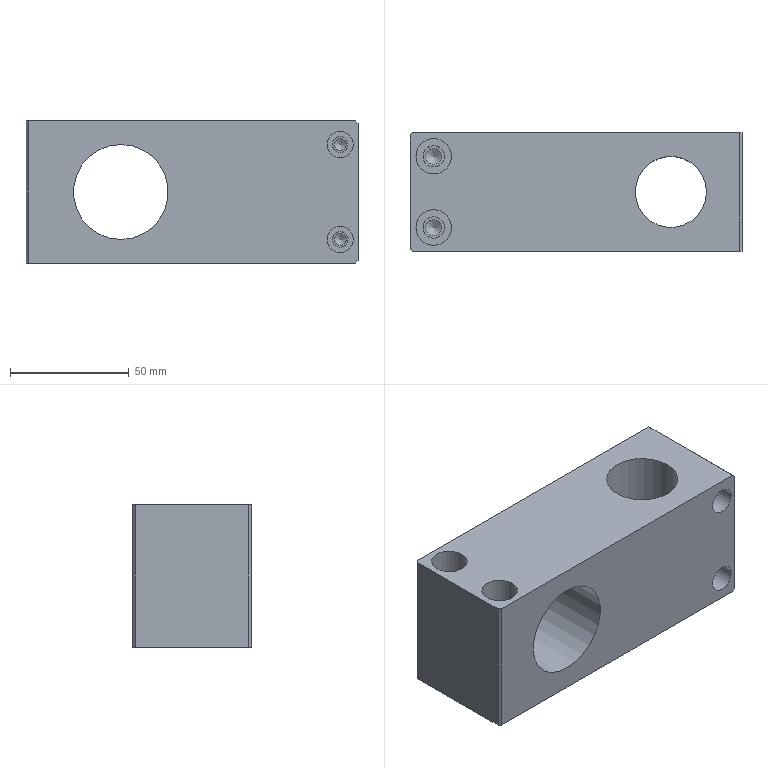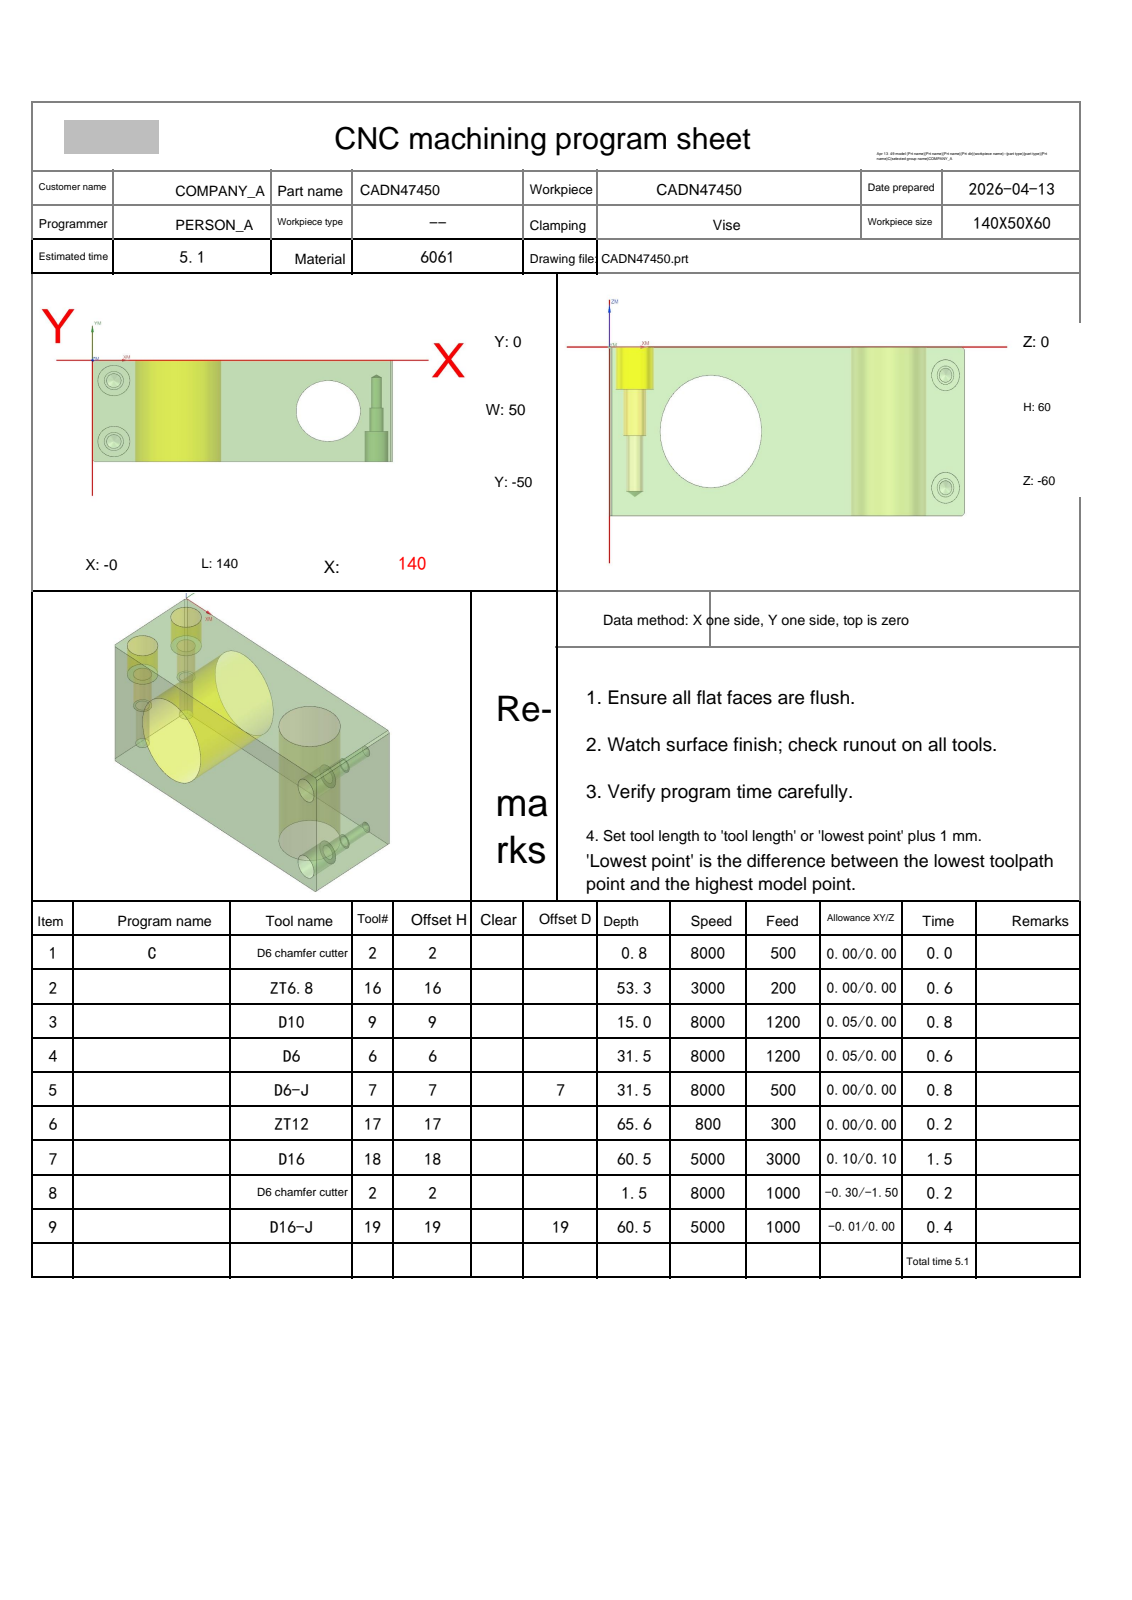NC program | NX | posted by the shop | part box 140 x 50 x 60 mm
Whole program:
%
O0001
(Machine time: 6.89 MIN)
(===Total Tool:8===)
(T2=D6 chamfer cutter   D=6.   R=0.   D-  H02 Z=-1.5  )
(T16=ZT6.8  D=6.8  DR_a=118 D-  H16 Z=-53.29)
(T9=D10     D=10.  R=0.   D-  H09 Z=-15.  )
(T6=D6      D=6.   R=0.   D-  H06 Z=-31.5 )
(T7=D6-J    D=6.   R=0.   D7  H07 Z=-31.5 )
(T17=ZT12   D=12.  DR_a=118 D-  H17 Z=-65.61)
(T18=D16    D=16.  R=0.   D-  H18 Z=-60.5 )
(T19=D16-J  D=16.  R=0.   D19 H19 Z=-60.5 )
G80 G90 G17 G49 G40
G91 G28 Z0
M01
N1 T02 M06
(D6 chamfer cutter  D=6. R=0. H=02 ce=0.00 di=0.00)
G00 G90 G54 X10. Y-40. M03 S8000
G43 H02 Z20.
M08
G98 G81 X10. Y-40. Z-.8 R1. F500.
Y-10.
X110. Y-25.
G80
G00 Z20.
G91 G28 Z0.0
M05
M09
G91 G28 Z0.0
M01
N2 T16 M06
(ZT6.8 D=6.8 DR_a=118 H=16)
G00 G90 G54 X10. Y-40. M03 S3000
G43 H16 Z20.
M08
G98 G83 X10. Y-40. Z-53.293 R1. F200. Q2.
Y-10.
G80
G00 Z20.
G91 G28 Z0.0
M05
M09
G91 G28 Z0.0
M01
N3 T09 M06
(D10  D=10. R=0. H=09 ce=0.05 di=0.00)
G00 G90 G54 X10. Y-40. M03 S8000
G43 H09 Z20.
M08
Z.5
G03 X11.225 Y-41.225 I1.225 J0.0 F1200.
X12.45 Y-40. I0.0 J1.225
X12.45 Y-40. Z0.0 I-2.45 J0.0
X12.45 Y-40. Z-.5 I-2.45 J0.0
X12.45 Y-40. Z-1. I-2.45 J0.0
X12.45 Y-40. Z-1.5 I-2.45 J0.0
X12.45 Y-40. Z-2. I-2.45 J0.0
X12.45 Y-40. Z-2.5 I-2.45 J0.0
X12.45 Y-40. Z-3. I-2.45 J0.0
X12.45 Y-40. Z-3.5 I-2.45 J0.0
X12.45 Y-40. Z-4. I-2.45 J0.0
X12.45 Y-40. Z-4.5 I-2.45 J0.0
X12.45 Y-40. Z-5. I-2.45 J0.0
X12.45 Y-40. Z-5.5 I-2.45 J0.0
X12.45 Y-40. Z-6. I-2.45 J0.0
X12.45 Y-40. Z-6.5 I-2.45 J0.0
X12.45 Y-40. Z-7. I-2.45 J0.0
X12.45 Y-40. Z-7.5 I-2.45 J0.0
X12.45 Y-40. Z-8. I-2.45 J0.0
X12.45 Y-40. Z-8.5 I-2.45 J0.0
X12.45 Y-40. Z-9. I-2.45 J0.0
X12.45 Y-40. Z-9.5 I-2.45 J0.0
X12.45 Y-40. Z-10. I-2.45 J0.0
X12.45 Y-40. Z-10.5 I-2.45 J0.0
X12.45 Y-40. Z-11. I-2.45 J0.0
X12.45 Y-40. Z-11.5 I-2.45 J0.0
X12.45 Y-40. Z-12. I-2.45 J0.0
X12.45 Y-40. Z-12.5 I-2.45 J0.0
X12.45 Y-40. Z-13. I-2.45 J0.0
X12.45 Y-40. Z-13.5 I-2.45 J0.0
X12.45 Y-40. Z-14. I-2.45 J0.0
X12.45 Y-40. Z-14.5 I-2.45 J0.0
X12.45 Y-40. Z-15. I-2.45 J0.0
X10. Y-37.55 I-2.45 J0.0
X7.55 Y-40. I0.0 J-2.45
X10. Y-42.45 I2.45 J0.0
X12.45 Y-40. I0.0 J2.45
X11.225 Y-38.775 I-1.225 J0.0
X10. Y-40. I0.0 J-1.225
G00 Z20.
Y-10.
Z.5
G03 X11.225 Y-11.225 I1.225 J0.0
X12.45 Y-10. I0.0 J1.225
X12.45 Y-10. Z0.0 I-2.45 J0.0
X12.45 Y-10. Z-.5 I-2.45 J0.0
X12.45 Y-10. Z-1. I-2.45 J0.0
X12.45 Y-10. Z-1.5 I-2.45 J0.0
X12.45 Y-10. Z-2. I-2.45 J0.0
X12.45 Y-10. Z-2.5 I-2.45 J0.0
X12.45 Y-10. Z-3. I-2.45 J0.0
X12.45 Y-10. Z-3.5 I-2.45 J0.0
X12.45 Y-10. Z-4. I-2.45 J0.0
X12.45 Y-10. Z-4.5 I-2.45 J0.0
X12.45 Y-10. Z-5. I-2.45 J0.0
X12.45 Y-10. Z-5.5 I-2.45 J0.0
X12.45 Y-10. Z-6. I-2.45 J0.0
X12.45 Y-10. Z-6.5 I-2.45 J0.0
X12.45 Y-10. Z-7. I-2.45 J0.0
X12.45 Y-10. Z-7.5 I-2.45 J0.0
X12.45 Y-10. Z-8. I-2.45 J0.0
X12.45 Y-10. Z-8.5 I-2.45 J0.0
X12.45 Y-10. Z-9. I-2.45 J0.0
X12.45 Y-10. Z-9.5 I-2.45 J0.0
X12.45 Y-10. Z-10. I-2.45 J0.0
X12.45 Y-10. Z-10.5 I-2.45 J0.0
X12.45 Y-10. Z-11. I-2.45 J0.0
X12.45 Y-10. Z-11.5 I-2.45 J0.0
X12.45 Y-10. Z-12. I-2.45 J0.0
X12.45 Y-10. Z-12.5 I-2.45 J0.0
X12.45 Y-10. Z-13. I-2.45 J0.0
X12.45 Y-10. Z-13.5 I-2.45 J0.0
X12.45 Y-10. Z-14. I-2.45 J0.0
X12.45 Y-10. Z-14.5 I-2.45 J0.0
X12.45 Y-10. Z-15. I-2.45 J0.0
X10. Y-7.55 I-2.45 J0.0
X7.55 Y-10. I0.0 J-2.45
X10. Y-12.45 I2.45 J0.0
X12.45 Y-10. I0.0 J2.45
X11.225 Y-8.775 I-1.225 J0.0
X10. Y-10. I0.0 J-1.225
G00 Z20.
G91 G28 Z0.0
M05
M09
G91 G28 Z0.0
M01
N4 T06 M06
(D6  D=6. R=0. H=06 ce=0.05 di=0.00)
G00 G90 G54 X10. Y-40. M03 S8000
G43 H06 Z20.
M08
Z-14.5
G03 X10.725 Y-40.725 I.725 J0.0 F1200.
X11.45 Y-40. I0.0 J.725
X11.45 Y-40. Z-15. I-1.45 J0.0
X11.45 Y-40. Z-15.5 I-1.45 J0.0
X11.45 Y-40. Z-16. I-1.45 J0.0
X11.45 Y-40. Z-16.5 I-1.45 J0.0
X11.45 Y-40. Z-17. I-1.45 J0.0
X11.45 Y-40. Z-17.5 I-1.45 J0.0
X11.45 Y-40. Z-18. I-1.45 J0.0
X11.45 Y-40. Z-18.5 I-1.45 J0.0
X11.45 Y-40. Z-19. I-1.45 J0.0
X11.45 Y-40. Z-19.5 I-1.45 J0.0
X11.45 Y-40. Z-20. I-1.45 J0.0
X11.45 Y-40. Z-20.5 I-1.45 J0.0
X11.45 Y-40. Z-21. I-1.45 J0.0
X11.45 Y-40. Z-21.5 I-1.45 J0.0
X11.45 Y-40. Z-22. I-1.45 J0.0
X11.45 Y-40. Z-22.5 I-1.45 J0.0
X11.45 Y-40. Z-23. I-1.45 J0.0
X11.45 Y-40. Z-23.5 I-1.45 J0.0
X11.45 Y-40. Z-24. I-1.45 J0.0
X11.45 Y-40. Z-24.5 I-1.45 J0.0
X11.45 Y-40. Z-25. I-1.45 J0.0
X11.45 Y-40. Z-25.5 I-1.45 J0.0
X11.45 Y-40. Z-26. I-1.45 J0.0
X11.45 Y-40. Z-26.5 I-1.45 J0.0
X11.45 Y-40. Z-27. I-1.45 J0.0
X11.45 Y-40. Z-27.5 I-1.45 J0.0
X11.45 Y-40. Z-28. I-1.45 J0.0
X11.45 Y-40. Z-28.5 I-1.45 J0.0
X11.45 Y-40. Z-29. I-1.45 J0.0
X11.45 Y-40. Z-29.5 I-1.45 J0.0
X11.45 Y-40. Z-30. I-1.45 J0.0
X11.45 Y-40. Z-30.5 I-1.45 J0.0
X11.45 Y-40. Z-31. I-1.45 J0.0
X11.45 Y-40. Z-31.5 I-1.45 J0.0
X10. Y-38.55 I-1.45 J0.0
X8.55 Y-40. I0.0 J-1.45
X10. Y-41.45 I1.45 J0.0
X11.45 Y-40. I0.0 J1.45
X10.725 Y-39.275 I-.725 J0.0
X10. Y-40. I0.0 J-.725
G00 Z20.
Y-10.
Z-14.5
G03 X10.725 Y-10.725 I.725 J0.0
X11.45 Y-10. I0.0 J.725
X11.45 Y-10. Z-15. I-1.45 J0.0
X11.45 Y-10. Z-15.5 I-1.45 J0.0
X11.45 Y-10. Z-16. I-1.45 J0.0
X11.45 Y-10. Z-16.5 I-1.45 J0.0
X11.45 Y-10. Z-17. I-1.45 J0.0
X11.45 Y-10. Z-17.5 I-1.45 J0.0
X11.45 Y-10. Z-18. I-1.45 J0.0
X11.45 Y-10. Z-18.5 I-1.45 J0.0
X11.45 Y-10. Z-19. I-1.45 J0.0
X11.45 Y-10. Z-19.5 I-1.45 J0.0
X11.45 Y-10. Z-20. I-1.45 J0.0
X11.45 Y-10. Z-20.5 I-1.45 J0.0
X11.45 Y-10. Z-21. I-1.45 J0.0
X11.45 Y-10. Z-21.5 I-1.45 J0.0
X11.45 Y-10. Z-22. I-1.45 J0.0
X11.45 Y-10. Z-22.5 I-1.45 J0.0
X11.45 Y-10. Z-23. I-1.45 J0.0
X11.45 Y-10. Z-23.5 I-1.45 J0.0
X11.45 Y-10. Z-24. I-1.45 J0.0
X11.45 Y-10. Z-24.5 I-1.45 J0.0
X11.45 Y-10. Z-25. I-1.45 J0.0
X11.45 Y-10. Z-25.5 I-1.45 J0.0
X11.45 Y-10. Z-26. I-1.45 J0.0
X11.45 Y-10. Z-26.5 I-1.45 J0.0
X11.45 Y-10. Z-27. I-1.45 J0.0
X11.45 Y-10. Z-27.5 I-1.45 J0.0
X11.45 Y-10. Z-28. I-1.45 J0.0
X11.45 Y-10. Z-28.5 I-1.45 J0.0
X11.45 Y-10. Z-29. I-1.45 J0.0
X11.45 Y-10. Z-29.5 I-1.45 J0.0
X11.45 Y-10. Z-30. I-1.45 J0.0
X11.45 Y-10. Z-30.5 I-1.45 J0.0
X11.45 Y-10. Z-31. I-1.45 J0.0
X11.45 Y-10. Z-31.5 I-1.45 J0.0
X10. Y-8.55 I-1.45 J0.0
X8.55 Y-10. I0.0 J-1.45
X10. Y-11.45 I1.45 J0.0
X11.45 Y-10. I0.0 J1.45
X10.725 Y-9.275 I-.725 J0.0
X10. Y-10. I0.0 J-.725
G00 Z20.
G91 G28 Z0.0
M05
M09
G91 G28 Z0.0
M01
N5 T07 M06
(D6-J  D=6. R=0. H=07 ce=0.00 di=0.00)
G00 G90 G54 X10. Y-40. M03 S8000
G43 H07 Z20.
M08
Z.5
G41 D07
G01 X10.847 Y-41.177 F500.
G03 X12.484 Y-42.016 I1.637 J1.177
X14.5 Y-40. I0.0 J2.016
X14.5 Y-40. Z-4.5 I-4.5 J0.0
X14.5 Y-40. Z-9.5 I-4.5 J0.0
X14.5 Y-40. Z-14.5 I-4.5 J0.0
X13.641 Y-37.355 Z-15. I-4.5 J0.0
X10. Y-35.5 I-3.641 J-2.645
X5.5 Y-40. I0.0 J-4.5
X10. Y-44.5 I4.5 J0.0
X14.5 Y-40. I0.0 J4.5
X13.641 Y-37.355 I-4.5 J0.0
X12.009 Y-36.524 I-1.631 J-1.185
X9.993 Y-38.54 I0.0 J-2.016
G01 Y-38.55
G40 X10. Y-40.
G00 Z20.
Y-10.
Z.5
G41 D07
G01 X10.847 Y-11.177
G03 X12.484 Y-12.016 I1.637 J1.177
X14.5 Y-10. I0.0 J2.016
X14.5 Y-10. Z-4.5 I-4.5 J0.0
X14.5 Y-10. Z-9.5 I-4.5 J0.0
X14.5 Y-10. Z-14.5 I-4.5 J0.0
X13.641 Y-7.355 Z-15. I-4.5 J0.0
X10. Y-5.5 I-3.641 J-2.645
X5.5 Y-10. I0.0 J-4.5
X10. Y-14.5 I4.5 J0.0
X14.5 Y-10. I0.0 J4.5
X13.641 Y-7.355 I-4.5 J0.0
X12.009 Y-6.524 I-1.631 J-1.185
X9.993 Y-8.54 I0.0 J-2.016
G01 Y-8.55
G40 X10. Y-10.
G00 Z20.
G00 G90 X10. Y-40. M03 S8000
Z20.
Z-14.5
G41 D07
G01 X10.052 Y-40.193 F500.
G03 X10.763 Y-40.737 I.711 J.193
X11.5 Y-40. I0.0 J.737
X11.5 Y-40. Z-19.5 I-1.5 J0.0
X11.5 Y-40. Z-24.5 I-1.5 J0.0
X11.5 Y-40. Z-29.5 I-1.5 J0.0
X8.786 Y-39.118 Z-31.5 I-1.5 J0.0
X8.5 Y-40. I1.214 J-.882
X10. Y-41.5 I1.5 J0.0
X11.5 Y-40. I0.0 J1.5
X10. Y-38.5 I-1.5 J0.0
X8.786 Y-39.118 I0.0 J-1.5
X8.646 Y-39.551 I.596 J-.433
X9.382 Y-40.288 I.737 J0.0
X9.844 Y-40.125 I0.0 J.737
G01 G40 X10. Y-40.
G00 Z20.
Y-10.
Z-14.5
G41 D07
G01 X10.052 Y-10.193
G03 X10.763 Y-10.737 I.711 J.193
X11.5 Y-10. I0.0 J.737
X11.5 Y-10. Z-19.5 I-1.5 J0.0
X11.5 Y-10. Z-24.5 I-1.5 J0.0
X11.5 Y-10. Z-29.5 I-1.5 J0.0
X8.786 Y-9.118 Z-31.5 I-1.5 J0.0
X8.5 Y-10. I1.214 J-.882
X10. Y-11.5 I1.5 J0.0
X11.5 Y-10. I0.0 J1.5
X10. Y-8.5 I-1.5 J0.0
X8.786 Y-9.118 I0.0 J-1.5
X8.646 Y-9.551 I.596 J-.433
X9.382 Y-10.288 I.737 J0.0
X9.844 Y-10.125 I0.0 J.737
G01 G40 X10. Y-10.
G00 Z20.
G91 G28 Z0.0
M05
M09
G91 G28 Z0.0
M01
N6 T17 M06
(ZT12 D=12. DR_a=118 H=17)
G00 G90 G54 X110. Y-25. M03 S800
G43 H17 Z20.
M08
G98 G83 X110. Y-25. Z-65.605 R1. F300. Q3.
G80
G00 Z20.
G91 G28 Z0.0
M05
M09
G91 G28 Z0.0
M01
N7 T18 M06
(D16  D=16. R=0. H=18 ce=0.10 di=0.10)
G00 G90 G54 X112.571 Y-31.398 M03 S5000
G43 H18 Z20.
M08
Z1.
G01 X113.65 Y-30.891 Z.938 F3000.
X114.9 Y-29.9 Z.854
X115.891 Y-28.65 Z.77
X116.57 Y-27.205 Z.687
X116.9 Y-25.644 Z.603
Y-24.356 Z.536
X116.57 Y-22.795 Z.452
X115.891 Y-21.35 Z.368
X114.9 Y-20.1 Z.285
X113.65 Y-19.109 Z.201
X112.205 Y-18.43 Z.117
X110.644 Y-18.1 Z.034
X110. Z0.0
G03 X103.1 Y-25. Z-.15 I0.0 J-6.9
X110. Y-31.9 Z-.3 I6.9 J0.0
X116.9 Y-25. Z-.449 I0.0 J6.9
X110. Y-18.1 Z-.599 I-6.9 J0.0
X103.1 Y-25. Z-.749 I0.0 J-6.9
X110. Y-31.9 Z-.899 I6.9 J0.0
X116.9 Y-25. Z-1.048 I0.0 J6.9
X110. Y-18.1 Z-1.198 I-6.9 J0.0
X103.1 Y-25. Z-1.348 I0.0 J-6.9
X110. Y-31.9 Z-1.498 I6.9 J0.0
X116.9 Y-25. Z-1.647 I0.0 J6.9
X110. Y-18.1 Z-1.797 I-6.9 J0.0
X103.1 Y-25. Z-1.947 I0.0 J-6.9
X110. Y-31.9 Z-2.097 I6.9 J0.0
X116.9 Y-25. Z-2.246 I0.0 J6.9
X110. Y-18.1 Z-2.396 I-6.9 J0.0
X103.1 Y-25. Z-2.546 I0.0 J-6.9
X110. Y-31.9 Z-2.696 I6.9 J0.0
X116.9 Y-25. Z-2.845 I0.0 J6.9
X110. Y-18.1 Z-2.995 I-6.9 J0.0
X103.1 Y-25. Z-3.145 I0.0 J-6.9
X110. Y-31.9 Z-3.295 I6.9 J0.0
X116.9 Y-25. Z-3.444 I0.0 J6.9
X110. Y-18.1 Z-3.594 I-6.9 J0.0
X103.1 Y-25. Z-3.744 I0.0 J-6.9
X110. Y-31.9 Z-3.894 I6.9 J0.0
X116.9 Y-25. Z-4.043 I0.0 J6.9
X110. Y-18.1 Z-4.193 I-6.9 J0.0
X103.1 Y-25. Z-4.343 I0.0 J-6.9
X110. Y-31.9 Z-4.493 I6.9 J0.0
X116.9 Y-25. Z-4.642 I0.0 J6.9
X110. Y-18.1 Z-4.792 I-6.9 J0.0
X103.1 Y-25. Z-4.942 I0.0 J-6.9
X110. Y-31.9 Z-5.092 I6.9 J0.0
X116.9 Y-25. Z-5.241 I0.0 J6.9
X110. Y-18.1 Z-5.391 I-6.9 J0.0
X103.1 Y-25. Z-5.541 I0.0 J-6.9
X110. Y-31.9 Z-5.691 I6.9 J0.0
X116.9 Y-25. Z-5.84 I0.0 J6.9
X110. Y-18.1 Z-5.99 I-6.9 J0.0
X103.1 Y-25. Z-6.14 I0.0 J-6.9
X110. Y-31.9 Z-6.29 I6.9 J0.0
X116.9 Y-25. Z-6.439 I0.0 J6.9
X110. Y-18.1 Z-6.589 I-6.9 J0.0
X103.1 Y-25. Z-6.739 I0.0 J-6.9
X110. Y-31.9 Z-6.889 I6.9 J0.0
X116.9 Y-25. Z-7.038 I0.0 J6.9
X110. Y-18.1 Z-7.188 I-6.9 J0.0
X103.1 Y-25. Z-7.338 I0.0 J-6.9
X110. Y-31.9 Z-7.488 I6.9 J0.0
X116.9 Y-25. Z-7.637 I0.0 J6.9
X110. Y-18.1 Z-7.787 I-6.9 J0.0
X103.1 Y-25. Z-7.937 I0.0 J-6.9
X110. Y-31.9 Z-8.087 I6.9 J0.0
X116.9 Y-25. Z-8.236 I0.0 J6.9
X110. Y-18.1 Z-8.386 I-6.9 J0.0
X103.1 Y-25. Z-8.536 I0.0 J-6.9
X110. Y-31.9 Z-8.686 I6.9 J0.0
X116.9 Y-25. Z-8.835 I0.0 J6.9
X110. Y-18.1 Z-8.985 I-6.9 J0.0
X103.1 Y-25. Z-9.135 I0.0 J-6.9
X110. Y-31.9 Z-9.285 I6.9 J0.0
X116.9 Y-25. Z-9.434 I0.0 J6.9
X110. Y-18.1 Z-9.584 I-6.9 J0.0
X103.1 Y-25. Z-9.734 I0.0 J-6.9
X110. Y-31.9 Z-9.884 I6.9 J0.0
X116.9 Y-25. Z-10.033 I0.0 J6.9
X110. Y-18.1 Z-10.183 I-6.9 J0.0
X103.1 Y-25. Z-10.333 I0.0 J-6.9
X110. Y-31.9 Z-10.483 I6.9 J0.0
X116.9 Y-25. Z-10.632 I0.0 J6.9
X110. Y-18.1 Z-10.782 I-6.9 J0.0
X103.1 Y-25. Z-10.932 I0.0 J-6.9
X110. Y-31.9 Z-11.082 I6.9 J0.0
X116.9 Y-25. Z-11.231 I0.0 J6.9
X110. Y-18.1 Z-11.381 I-6.9 J0.0
X103.1 Y-25. Z-11.531 I0.0 J-6.9
X110. Y-31.9 Z-11.681 I6.9 J0.0
X116.9 Y-25. Z-11.83 I0.0 J6.9
X110. Y-18.1 Z-11.98 I-6.9 J0.0
X103.1 Y-25. Z-12.13 I0.0 J-6.9
X110. Y-31.9 Z-12.28 I6.9 J0.0
X116.9 Y-25. Z-12.429 I0.0 J6.9
X110. Y-18.1 Z-12.579 I-6.9 J0.0
X103.1 Y-25. Z-12.729 I0.0 J-6.9
X110. Y-31.9 Z-12.879 I6.9 J0.0
X116.9 Y-25. Z-13.028 I0.0 J6.9
X110. Y-18.1 Z-13.178 I-6.9 J0.0
X103.1 Y-25. Z-13.328 I0.0 J-6.9
X110. Y-31.9 Z-13.478 I6.9 J0.0
X116.9 Y-25. Z-13.627 I0.0 J6.9
X110. Y-18.1 Z-13.777 I-6.9 J0.0
X103.1 Y-25. Z-13.927 I0.0 J-6.9
X110. Y-31.9 Z-14.077 I6.9 J0.0
X116.9 Y-25. Z-14.226 I0.0 J6.9
X110. Y-18.1 Z-14.376 I-6.9 J0.0
X103.1 Y-25. Z-14.526 I0.0 J-6.9
X110. Y-31.9 Z-14.676 I6.9 J0.0
X116.9 Y-25. Z-14.825 I0.0 J6.9
X110. Y-18.1 Z-14.975 I-6.9 J0.0
X103.1 Y-25. Z-15.125 I0.0 J-6.9
X110. Y-31.9 Z-15.275 I6.9 J0.0
X116.9 Y-25. Z-15.425 I0.0 J6.9
X110. Y-18.1 Z-15.574 I-6.9 J0.0
X103.1 Y-25. Z-15.724 I0.0 J-6.9
X110. Y-31.9 Z-15.874 I6.9 J0.0
X116.9 Y-25. Z-16.024 I0.0 J6.9
X110. Y-18.1 Z-16.173 I-6.9 J0.0
X103.1 Y-25. Z-16.323 I0.0 J-6.9
X110. Y-31.9 Z-16.473 I6.9 J0.0
X116.9 Y-25. Z-16.623 I0.0 J6.9
X110. Y-18.1 Z-16.772 I-6.9 J0.0
X103.1 Y-25. Z-16.922 I0.0 J-6.9
X110. Y-31.9 Z-17.072 I6.9 J0.0
X116.9 Y-25. Z-17.222 I0.0 J6.9
X110. Y-18.1 Z-17.371 I-6.9 J0.0
X103.1 Y-25. Z-17.521 I0.0 J-6.9
X110. Y-31.9 Z-17.671 I6.9 J0.0
X116.9 Y-25. Z-17.821 I0.0 J6.9
X110. Y-18.1 Z-17.97 I-6.9 J0.0
X103.1 Y-25. Z-18.12 I0.0 J-6.9
X110. Y-31.9 Z-18.27 I6.9 J0.0
X116.9 Y-25. Z-18.42 I0.0 J6.9
X110. Y-18.1 Z-18.569 I-6.9 J0.0
X103.1 Y-25. Z-18.719 I0.0 J-6.9
X110. Y-31.9 Z-18.869 I6.9 J0.0
X116.9 Y-25. Z-19.019 I0.0 J6.9
X110. Y-18.1 Z-19.168 I-6.9 J0.0
X103.1 Y-25. Z-19.318 I0.0 J-6.9
X110. Y-31.9 Z-19.468 I6.9 J0.0
X116.9 Y-25. Z-19.618 I0.0 J6.9
X110. Y-18.1 Z-19.767 I-6.9 J0.0
X103.1 Y-25. Z-19.917 I0.0 J-6.9
X110. Y-31.9 Z-20.067 I6.9 J0.0
X116.9 Y-25. Z-20.217 I0.0 J6.9
X110. Y-18.1 Z-20.366 I-6.9 J0.0
X103.1 Y-25. Z-20.516 I0.0 J-6.9
X110. Y-31.9 Z-20.666 I6.9 J0.0
X116.9 Y-25. Z-20.816 I0.0 J6.9
X110. Y-18.1 Z-20.965 I-6.9 J0.0
X103.1 Y-25. Z-21.115 I0.0 J-6.9
X110. Y-31.9 Z-21.265 I6.9 J0.0
X116.9 Y-25. Z-21.415 I0.0 J6.9
X110. Y-18.1 Z-21.564 I-6.9 J0.0
X103.1 Y-25. Z-21.714 I0.0 J-6.9
X110. Y-31.9 Z-21.864 I6.9 J0.0
X116.9 Y-25. Z-22.014 I0.0 J6.9
X110. Y-18.1 Z-22.163 I-6.9 J0.0
X103.1 Y-25. Z-22.313 I0.0 J-6.9
X110. Y-31.9 Z-22.463 I6.9 J0.0
X116.9 Y-25. Z-22.613 I0.0 J6.9
X110. Y-18.1 Z-22.762 I-6.9 J0.0
X103.1 Y-25. Z-22.912 I0.0 J-6.9
X110. Y-31.9 Z-23.062 I6.9 J0.0
X116.9 Y-25. Z-23.212 I0.0 J6.9
X110. Y-18.1 Z-23.361 I-6.9 J0.0
X103.1 Y-25. Z-23.511 I0.0 J-6.9
X110. Y-31.9 Z-23.661 I6.9 J0.0
X116.9 Y-25. Z-23.811 I0.0 J6.9
X110. Y-18.1 Z-23.96 I-6.9 J0.0
X103.1 Y-25. Z-24.11 I0.0 J-6.9
X110. Y-31.9 Z-24.26 I6.9 J0.0
X116.9 Y-25. Z-24.41 I0.0 J6.9
X110. Y-18.1 Z-24.559 I-6.9 J0.0
X103.1 Y-25. Z-24.709 I0.0 J-6.9
X110. Y-31.9 Z-24.859 I6.9 J0.0
X116.9 Y-25. Z-25.009 I0.0 J6.9
X110. Y-18.1 Z-25.158 I-6.9 J0.0
X103.1 Y-25. Z-25.308 I0.0 J-6.9
X110. Y-31.9 Z-25.458 I6.9 J0.0
X116.9 Y-25. Z-25.608 I0.0 J6.9
X110. Y-18.1 Z-25.757 I-6.9 J0.0
X103.1 Y-25. Z-25.907 I0.0 J-6.9
X110. Y-31.9 Z-26.057 I6.9 J0.0
X116.9 Y-25. Z-26.207 I0.0 J6.9
X110. Y-18.1 Z-26.356 I-6.9 J0.0
X103.1 Y-25. Z-26.506 I0.0 J-6.9
X110. Y-31.9 Z-26.656 I6.9 J0.0
X116.9 Y-25. Z-26.806 I0.0 J6.9
X110. Y-18.1 Z-26.955 I-6.9 J0.0
X103.1 Y-25. Z-27.105 I0.0 J-6.9
X110. Y-31.9 Z-27.255 I6.9 J0.0
X116.9 Y-25. Z-27.405 I0.0 J6.9
X110. Y-18.1 Z-27.554 I-6.9 J0.0
X103.1 Y-25. Z-27.704 I0.0 J-6.9
X110. Y-31.9 Z-27.854 I6.9 J0.0
X116.9 Y-25. Z-28.004 I0.0 J6.9
X110. Y-18.1 Z-28.153 I-6.9 J0.0
X103.1 Y-25. Z-28.303 I0.0 J-6.9
X110. Y-31.9 Z-28.453 I6.9 J0.0
X116.9 Y-25. Z-28.603 I0.0 J6.9
X110. Y-18.1 Z-28.752 I-6.9 J0.0
X103.1 Y-25. Z-28.902 I0.0 J-6.9
X110. Y-31.9 Z-29.052 I6.9 J0.0
X116.9 Y-25. Z-29.202 I0.0 J6.9
X110. Y-18.1 Z-29.351 I-6.9 J0.0
X103.1 Y-25. Z-29.501 I0.0 J-6.9
X110. Y-31.9 Z-29.651 I6.9 J0.0
X116.9 Y-25. Z-29.801 I0.0 J6.9
X110. Y-18.1 Z-29.95 I-6.9 J0.0
X103.1 Y-25. Z-30.1 I0.0 J-6.9
X110. Y-31.9 Z-30.25 I6.9 J0.0
X116.9 Y-25. Z-30.4 I0.0 J6.9
X110. Y-18.1 Z-30.55 I-6.9 J0.0
X103.1 Y-25. Z-30.699 I0.0 J-6.9
X110. Y-31.9 Z-30.849 I6.9 J0.0
X116.9 Y-25. Z-30.999 I0.0 J6.9
X110. Y-18.1 Z-31.149 I-6.9 J0.0
X103.1 Y-25. Z-31.298 I0.0 J-6.9
X110. Y-31.9 Z-31.448 I6.9 J0.0
X116.9 Y-25. Z-31.598 I0.0 J6.9
X110. Y-18.1 Z-31.748 I-6.9 J0.0
X103.1 Y-25. Z-31.897 I0.0 J-6.9
X110. Y-31.9 Z-32.047 I6.9 J0.0
X116.9 Y-25. Z-32.197 I0.0 J6.9
X110. Y-18.1 Z-32.347 I-6.9 J0.0
X103.1 Y-25. Z-32.496 I0.0 J-6.9
X110. Y-31.9 Z-32.646 I6.9 J0.0
X116.9 Y-25. Z-32.796 I0.0 J6.9
X110. Y-18.1 Z-32.946 I-6.9 J0.0
X103.1 Y-25. Z-33.095 I0.0 J-6.9
X110. Y-31.9 Z-33.245 I6.9 J0.0
X116.9 Y-25. Z-33.395 I0.0 J6.9
X110. Y-18.1 Z-33.545 I-6.9 J0.0
X103.1 Y-25. Z-33.694 I0.0 J-6.9
X110. Y-31.9 Z-33.844 I6.9 J0.0
X116.9 Y-25. Z-33.994 I0.0 J6.9
X110. Y-18.1 Z-34.144 I-6.9 J0.0
X103.1 Y-25. Z-34.293 I0.0 J-6.9
X110. Y-31.9 Z-34.443 I6.9 J0.0
X116.9 Y-25. Z-34.593 I0.0 J6.9
X110. Y-18.1 Z-34.743 I-6.9 J0.0
X103.1 Y-25. Z-34.892 I0.0 J-6.9
X110. Y-31.9 Z-35.042 I6.9 J0.0
X116.9 Y-25. Z-35.192 I0.0 J6.9
X110. Y-18.1 Z-35.342 I-6.9 J0.0
X103.1 Y-25. Z-35.491 I0.0 J-6.9
X110. Y-31.9 Z-35.641 I6.9 J0.0
X116.9 Y-25. Z-35.791 I0.0 J6.9
X110. Y-18.1 Z-35.941 I-6.9 J0.0
X103.1 Y-25. Z-36.09 I0.0 J-6.9
X110. Y-31.9 Z-36.24 I6.9 J0.0
X116.9 Y-25. Z-36.39 I0.0 J6.9
X110. Y-18.1 Z-36.54 I-6.9 J0.0
X103.1 Y-25. Z-36.689 I0.0 J-6.9
X110. Y-31.9 Z-36.839 I6.9 J0.0
X116.9 Y-25. Z-36.989 I0.0 J6.9
X110. Y-18.1 Z-37.139 I-6.9 J0.0
X103.1 Y-25. Z-37.288 I0.0 J-6.9
X110. Y-31.9 Z-37.438 I6.9 J0.0
X116.9 Y-25. Z-37.588 I0.0 J6.9
X110. Y-18.1 Z-37.738 I-6.9 J0.0
X103.1 Y-25. Z-37.887 I0.0 J-6.9
X110. Y-31.9 Z-38.037 I6.9 J0.0
X116.9 Y-25. Z-38.187 I0.0 J6.9
X110. Y-18.1 Z-38.337 I-6.9 J0.0
X103.1 Y-25. Z-38.486 I0.0 J-6.9
X110. Y-31.9 Z-38.636 I6.9 J0.0
X116.9 Y-25. Z-38.786 I0.0 J6.9
X110. Y-18.1 Z-38.936 I-6.9 J0.0
X103.1 Y-25. Z-39.085 I0.0 J-6.9
X110. Y-31.9 Z-39.235 I6.9 J0.0
X116.9 Y-25. Z-39.385 I0.0 J6.9
X110. Y-18.1 Z-39.535 I-6.9 J0.0
X103.1 Y-25. Z-39.684 I0.0 J-6.9
X110. Y-31.9 Z-39.834 I6.9 J0.0
X116.9 Y-25. Z-39.984 I0.0 J6.9
X110. Y-18.1 Z-40.134 I-6.9 J0.0
X103.1 Y-25. Z-40.283 I0.0 J-6.9
X110. Y-31.9 Z-40.433 I6.9 J0.0
X116.9 Y-25. Z-40.583 I0.0 J6.9
X110. Y-18.1 Z-40.733 I-6.9 J0.0
X103.1 Y-25. Z-40.882 I0.0 J-6.9
X110. Y-31.9 Z-41.032 I6.9 J0.0
X116.9 Y-25. Z-41.182 I0.0 J6.9
X110. Y-18.1 Z-41.332 I-6.9 J0.0
X103.1 Y-25. Z-41.481 I0.0 J-6.9
X110. Y-31.9 Z-41.631 I6.9 J0.0
X116.9 Y-25. Z-41.781 I0.0 J6.9
X110. Y-18.1 Z-41.931 I-6.9 J0.0
X103.1 Y-25. Z-42.08 I0.0 J-6.9
X110. Y-31.9 Z-42.23 I6.9 J0.0
X116.9 Y-25. Z-42.38 I0.0 J6.9
X110. Y-18.1 Z-42.53 I-6.9 J0.0
X103.1 Y-25. Z-42.679 I0.0 J-6.9
X110. Y-31.9 Z-42.829 I6.9 J0.0
X116.9 Y-25. Z-42.979 I0.0 J6.9
X110. Y-18.1 Z-43.129 I-6.9 J0.0
X103.1 Y-25. Z-43.278 I0.0 J-6.9
X110. Y-31.9 Z-43.428 I6.9 J0.0
X116.9 Y-25. Z-43.578 I0.0 J6.9
X110. Y-18.1 Z-43.728 I-6.9 J0.0
X103.1 Y-25. Z-43.877 I0.0 J-6.9
X110. Y-31.9 Z-44.027 I6.9 J0.0
X116.9 Y-25. Z-44.177 I0.0 J6.9
X110. Y-18.1 Z-44.327 I-6.9 J0.0
X103.1 Y-25. Z-44.476 I0.0 J-6.9
X110. Y-31.9 Z-44.626 I6.9 J0.0
X116.9 Y-25. Z-44.776 I0.0 J6.9
X110. Y-18.1 Z-44.926 I-6.9 J0.0
X103.1 Y-25. Z-45.075 I0.0 J-6.9
X110. Y-31.9 Z-45.225 I6.9 J0.0
X116.9 Y-25. Z-45.375 I0.0 J6.9
X110. Y-18.1 Z-45.525 I-6.9 J0.0
X103.1 Y-25. Z-45.675 I0.0 J-6.9
X110. Y-31.9 Z-45.824 I6.9 J0.0
X116.9 Y-25. Z-45.974 I0.0 J6.9
X110. Y-18.1 Z-46.124 I-6.9 J0.0
X103.1 Y-25. Z-46.274 I0.0 J-6.9
X110. Y-31.9 Z-46.423 I6.9 J0.0
X116.9 Y-25. Z-46.573 I0.0 J6.9
X110. Y-18.1 Z-46.723 I-6.9 J0.0
X103.1 Y-25. Z-46.873 I0.0 J-6.9
X110. Y-31.9 Z-47.022 I6.9 J0.0
X116.9 Y-25. Z-47.172 I0.0 J6.9
X110. Y-18.1 Z-47.322 I-6.9 J0.0
X103.1 Y-25. Z-47.472 I0.0 J-6.9
X110. Y-31.9 Z-47.621 I6.9 J0.0
X116.9 Y-25. Z-47.771 I0.0 J6.9
X110. Y-18.1 Z-47.921 I-6.9 J0.0
X103.1 Y-25. Z-48.071 I0.0 J-6.9
X110. Y-31.9 Z-48.22 I6.9 J0.0
X116.9 Y-25. Z-48.37 I0.0 J6.9
X110. Y-18.1 Z-48.52 I-6.9 J0.0
X103.1 Y-25. Z-48.67 I0.0 J-6.9
X110. Y-31.9 Z-48.819 I6.9 J0.0
X116.9 Y-25. Z-48.969 I0.0 J6.9
X110. Y-18.1 Z-49.119 I-6.9 J0.0
X103.1 Y-25. Z-49.269 I0.0 J-6.9
X110. Y-31.9 Z-49.418 I6.9 J0.0
X116.9 Y-25. Z-49.568 I0.0 J6.9
X110. Y-18.1 Z-49.718 I-6.9 J0.0
X103.1 Y-25. Z-49.868 I0.0 J-6.9
X110. Y-31.9 Z-50.017 I6.9 J0.0
X116.9 Y-25. Z-50.167 I0.0 J6.9
X110. Y-18.1 Z-50.317 I-6.9 J0.0
X103.1 Y-25. Z-50.467 I0.0 J-6.9
X110. Y-31.9 Z-50.616 I6.9 J0.0
X116.9 Y-25. Z-50.766 I0.0 J6.9
X110. Y-18.1 Z-50.916 I-6.9 J0.0
X103.1 Y-25. Z-51.066 I0.0 J-6.9
X110. Y-31.9 Z-51.215 I6.9 J0.0
X116.9 Y-25. Z-51.365 I0.0 J6.9
X110. Y-18.1 Z-51.515 I-6.9 J0.0
X103.1 Y-25. Z-51.665 I0.0 J-6.9
X110. Y-31.9 Z-51.814 I6.9 J0.0
X116.9 Y-25. Z-51.964 I0.0 J6.9
X110. Y-18.1 Z-52.114 I-6.9 J0.0
X103.1 Y-25. Z-52.264 I0.0 J-6.9
X110. Y-31.9 Z-52.413 I6.9 J0.0
X116.9 Y-25. Z-52.563 I0.0 J6.9
X110. Y-18.1 Z-52.713 I-6.9 J0.0
X103.1 Y-25. Z-52.863 I0.0 J-6.9
X110. Y-31.9 Z-53.012 I6.9 J0.0
X116.9 Y-25. Z-53.162 I0.0 J6.9
X110. Y-18.1 Z-53.312 I-6.9 J0.0
X103.1 Y-25. Z-53.462 I0.0 J-6.9
X110. Y-31.9 Z-53.611 I6.9 J0.0
X116.9 Y-25. Z-53.761 I0.0 J6.9
X110. Y-18.1 Z-53.911 I-6.9 J0.0
X103.1 Y-25. Z-54.061 I0.0 J-6.9
X110. Y-31.9 Z-54.21 I6.9 J0.0
X116.9 Y-25. Z-54.36 I0.0 J6.9
X110. Y-18.1 Z-54.51 I-6.9 J0.0
X103.1 Y-25. Z-54.66 I0.0 J-6.9
X110. Y-31.9 Z-54.809 I6.9 J0.0
X116.9 Y-25. Z-54.959 I0.0 J6.9
X110. Y-18.1 Z-55.109 I-6.9 J0.0
X103.1 Y-25. Z-55.259 I0.0 J-6.9
X110. Y-31.9 Z-55.408 I6.9 J0.0
X116.9 Y-25. Z-55.558 I0.0 J6.9
X110. Y-18.1 Z-55.708 I-6.9 J0.0
X103.1 Y-25. Z-55.858 I0.0 J-6.9
X110. Y-31.9 Z-56.007 I6.9 J0.0
X116.9 Y-25. Z-56.157 I0.0 J6.9
X110. Y-18.1 Z-56.307 I-6.9 J0.0
X103.1 Y-25. Z-56.457 I0.0 J-6.9
X110. Y-31.9 Z-56.606 I6.9 J0.0
X116.9 Y-25. Z-56.756 I0.0 J6.9
X110. Y-18.1 Z-56.906 I-6.9 J0.0
X103.1 Y-25. Z-57.056 I0.0 J-6.9
X110. Y-31.9 Z-57.205 I6.9 J0.0
X116.9 Y-25. Z-57.355 I0.0 J6.9
X110. Y-18.1 Z-57.505 I-6.9 J0.0
X103.1 Y-25. Z-57.655 I0.0 J-6.9
X110. Y-31.9 Z-57.804 I6.9 J0.0
X116.9 Y-25. Z-57.954 I0.0 J6.9
X110. Y-18.1 Z-58.104 I-6.9 J0.0
X103.1 Y-25. Z-58.254 I0.0 J-6.9
X110. Y-31.9 Z-58.403 I6.9 J0.0
X116.9 Y-25. Z-58.553 I0.0 J6.9
X110. Y-18.1 Z-58.703 I-6.9 J0.0
X103.1 Y-25. Z-58.853 I0.0 J-6.9
X110. Y-31.9 Z-59.002 I6.9 J0.0
X116.9 Y-25. Z-59.152 I0.0 J6.9
X110. Y-18.1 Z-59.302 I-6.9 J0.0
X103.1 Y-25. Z-59.452 I0.0 J-6.9
X110. Y-31.9 Z-59.601 I6.9 J0.0
X116.9 Y-25. Z-59.751 I0.0 J6.9
X110. Y-18.1 Z-59.901 I-6.9 J0.0
X103.1 Y-25. Z-60.051 I0.0 J-6.9
X110. Y-31.9 Z-60.2 I6.9 J0.0
X116.9 Y-25. Z-60.35 I0.0 J6.9
X110. Y-18.1 Z-60.5 I-6.9 J0.0
X103.1 Y-25. I0.0 J-6.9
X110. Y-31.9 I6.9 J0.0
X116.9 Y-25. I0.0 J6.9
X110. Y-18.1 I-6.9 J0.0
X109.6 Y-18.112 I0.0 J-6.9
G01 Z-59.5
G00 Z20.
G91 G28 Z0.0
M05
M09
G91 G28 Z0.0
M01
N8 T02 M06
(D6 chamfer cutter  D=6. R=0. H=02 ce=-0.30 di=0.00)
G00 G90 G54 X6.2 Y-37. M03 S8000
G43 H02 Z20.
M08
Z-.5
G01 Z-1. F800.
G03 X3.2 Y-40. I0.0 J-3.
X10. Y-46.8 I6.8 J0.0
X16.8 Y-40. I0.0 J6.8
X10. Y-33.2 I-6.8 J0.0
X3.2 Y-40. I0.0 J-6.8
X6.2 Y-43. I3. J0.0
G01 Z-.5
G00 Z20.
Y-7.
Z-.5
G01 Z-1.
G03 X3.2 Y-10. I0.0 J-3.
X10. Y-16.8 I6.8 J0.0
X16.8 Y-10. I0.0 J6.8
X10. Y-3.2 I-6.8 J0.0
X3.2 Y-10. I0.0 J-6.8
X6.2 Y-13. I3. J0.0
G01 Z-.5
G00 Z20.
G00 G90 X99.2 Y-22. M03 S8000
Z20.
Z-1.
G01 Z-1.5 F1000.
G03 X96.2 Y-25. I0.0 J-3.
X110. Y-38.8 I13.8 J0.0
X123.8 Y-25. I0.0 J13.8
X110. Y-11.2 I-13.8 J0.0
X96.2 Y-25. I0.0 J-13.8
X99.2 Y-28. I3. J0.0
G01 Z-1.
G00 Z20.
G91 G28 Z0.0
M05
M09
G91 G28 Z0.0
M01
N9 T19 M06
(D16-J  D=16. R=0. H=19 ce=-0.01 di=0.00)
G00 G90 G54 X107.6 Y-28.736 M03 S5000
G43 H19 Z10.
M08
Z-7.143
G01 Z-8.643 F1000.
G41 D19
Y-29.61
G03 X110. Y-32.01 I2.4 J0.0
X117.01 Y-25. I0.0 J7.01
X110. Y-17.99 I-7.01 J0.0
X102.99 Y-25. I0.0 J-7.01
X110. Y-32.01 I7.01 J0.0
X110.4 Y-31.999 I0.0 J7.01
X112.663 Y-29.602 I-.137 J2.396
G01 X112.659 Y-29.466
X112.621 Y-28.793
G40 X112.609 Y-28.593
Z-7.143
G00 X107.6 Y-28.736
Z-15.786
G01 Z-17.286
G41 D19
Y-29.61
G03 X110. Y-32.01 I2.4 J0.0
X117.01 Y-25. I0.0 J7.01
X110. Y-17.99 I-7.01 J0.0
X102.99 Y-25. I0.0 J-7.01
X110. Y-32.01 I7.01 J0.0
X110.4 Y-31.999 I0.0 J7.01
X112.663 Y-29.602 I-.137 J2.396
G01 X112.659 Y-29.466
X112.621 Y-28.793
G40 X112.609 Y-28.593
Z-15.786
G00 X107.6 Y-28.736
Z-24.429
G01 Z-25.929
G41 D19
Y-29.61
G03 X110. Y-32.01 I2.4 J0.0
X117.01 Y-25. I0.0 J7.01
X110. Y-17.99 I-7.01 J0.0
X102.99 Y-25. I0.0 J-7.01
X110. Y-32.01 I7.01 J0.0
X110.4 Y-31.999 I0.0 J7.01
X112.663 Y-29.602 I-.137 J2.396
G01 X112.659 Y-29.466
X112.621 Y-28.793
G40 X112.609 Y-28.593
Z-24.429
G00 X107.6 Y-28.736
Z-33.071
G01 Z-34.571
G41 D19
Y-29.61
G03 X110. Y-32.01 I2.4 J0.0
X117.01 Y-25. I0.0 J7.01
X110. Y-17.99 I-7.01 J0.0
X102.99 Y-25. I0.0 J-7.01
X110. Y-32.01 I7.01 J0.0
X110.4 Y-31.999 I0.0 J7.01
X112.663 Y-29.602 I-.137 J2.396
G01 X112.659 Y-29.466
X112.621 Y-28.793
G40 X112.609 Y-28.593
Z-33.071
G00 X107.6 Y-28.736
Z-41.714
G01 Z-43.214
G41 D19
Y-29.61
G03 X110. Y-32.01 I2.4 J0.0
X117.01 Y-25. I0.0 J7.01
X110. Y-17.99 I-7.01 J0.0
X102.99 Y-25. I0.0 J-7.01
X110. Y-32.01 I7.01 J0.0
X110.4 Y-31.999 I0.0 J7.01
X112.663 Y-29.602 I-.137 J2.396
G01 X112.659 Y-29.466
X112.621 Y-28.793
G40 X112.609 Y-28.593
Z-41.714
G00 X107.6 Y-28.736
Z-50.357
G01 Z-51.857
G41 D19
Y-29.61
G03 X110. Y-32.01 I2.4 J0.0
X117.01 Y-25. I0.0 J7.01
X110. Y-17.99 I-7.01 J0.0
X102.99 Y-25. I0.0 J-7.01
X110. Y-32.01 I7.01 J0.0
X110.4 Y-31.999 I0.0 J7.01
X112.663 Y-29.602 I-.137 J2.396
G01 X112.659 Y-29.466
X112.621 Y-28.793
G40 X112.609 Y-28.593
Z-50.357
G00 X107.6 Y-28.736
Z-59.
G01 Z-60.5
G41 D19
Y-29.61
G03 X110. Y-32.01 I2.4 J0.0
X117.01 Y-25. I0.0 J7.01
X110. Y-17.99 I-7.01 J0.0
X102.99 Y-25. I0.0 J-7.01
X110. Y-32.01 I7.01 J0.0
X110.4 Y-31.999 I0.0 J7.01
X112.663 Y-29.602 I-.137 J2.396
G01 X112.659 Y-29.466
X112.621 Y-28.793
G40 X112.609 Y-28.593
Z-59.
G00 Z10.
M05
M09
G91 G28 Z0.0
G91 G28 Y0.0
M30
%